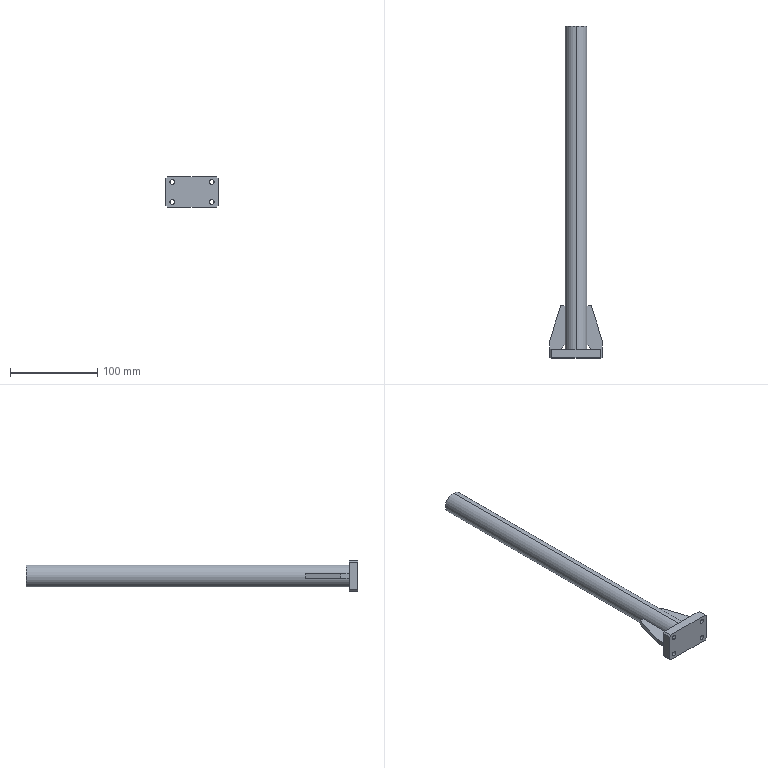Part | SolidWorks | features HoleWzd 2, ICE 2, Chamfer 1, Extrusion 1 | 4 solids | 42 faces | box 60 x 380 x 35 mm | volume 206976 mm3 | plane 28 | cylinder 12 | cone 2 | commonest cylinder face diameters 5.5 x8 6.8 x2 25 x2
STEP:
#1=CARTESIAN_POINT('',(17.5,0.,-2.5));
#2=VERTEX_POINT('',#1);
#3=CARTESIAN_POINT('',(30.,0.,-2.5));
#4=VERTEX_POINT('',#3);
#5=CARTESIAN_POINT('',(17.5,0.,-2.5));
#6=DIRECTION('',(1.,0.,0.));
#7=VECTOR('',#6,1000.);
#8=LINE('',#5,#7);
#9=EDGE_CURVE('',#2,#4,#8,.T.);
#10=ORIENTED_EDGE('',*,*,#9,.T.);
#11=CARTESIAN_POINT('',(30.,0.,2.5));
#12=VERTEX_POINT('',#11);
#13=CARTESIAN_POINT('',(30.,0.,2.5));
#14=DIRECTION('',(0.,0.,-1.));
#15=VECTOR('',#14,1000.);
#16=LINE('',#13,#15);
#17=EDGE_CURVE('',#12,#4,#16,.T.);
#18=ORIENTED_EDGE('',*,*,#17,.F.);
#19=CARTESIAN_POINT('',(17.5,0.,2.5));
#20=VERTEX_POINT('',#19);
#21=CARTESIAN_POINT('',(17.5,0.,2.5));
#22=DIRECTION('',(1.,0.,0.));
#23=VECTOR('',#22,1000.);
#24=LINE('',#21,#23);
#25=EDGE_CURVE('',#20,#12,#24,.T.);
#26=ORIENTED_EDGE('',*,*,#25,.F.);
#27=CARTESIAN_POINT('',(17.5,0.,2.5));
#28=DIRECTION('',(0.,0.,-1.));
#29=VECTOR('',#28,1000.);
#30=LINE('',#27,#29);
#31=EDGE_CURVE('',#20,#2,#30,.T.);
#32=ORIENTED_EDGE('',*,*,#31,.T.);
#33=EDGE_LOOP('',(#10,#18,#26,#32));
#34=FACE_OUTER_BOUND('',#33,.T.);
#35=CARTESIAN_POINT('',(17.5,0.,2.5));
#36=DIRECTION('',(0.,1.,0.));
#37=DIRECTION('',(0.,0.,1.));
#38=AXIS2_PLACEMENT_3D('',#35,#36,#37);
#39=PLANE('',#38);
#40=ADVANCED_FACE('',(#34),#39,.F.);
#41=CARTESIAN_POINT('',(30.,10.,-2.5));
#42=VERTEX_POINT('',#41);
#43=CARTESIAN_POINT('',(30.,0.,-2.5));
#44=DIRECTION('',(0.,1.,0.));
#45=VECTOR('',#44,1000.);
#46=LINE('',#43,#45);
#47=EDGE_CURVE('',#4,#42,#46,.T.);
#48=ORIENTED_EDGE('',*,*,#47,.T.);
#49=CARTESIAN_POINT('',(30.,10.,2.5));
#50=VERTEX_POINT('',#49);
#51=CARTESIAN_POINT('',(30.,10.,2.5));
#52=DIRECTION('',(0.,0.,-1.));
#53=VECTOR('',#52,1000.);
#54=LINE('',#51,#53);
#55=EDGE_CURVE('',#50,#42,#54,.T.);
#56=ORIENTED_EDGE('',*,*,#55,.F.);
#57=CARTESIAN_POINT('',(30.,0.,2.5));
#58=DIRECTION('',(0.,1.,0.));
#59=VECTOR('',#58,1000.);
#60=LINE('',#57,#59);
#61=EDGE_CURVE('',#12,#50,#60,.T.);
#62=ORIENTED_EDGE('',*,*,#61,.F.);
#63=ORIENTED_EDGE('',*,*,#17,.T.);
#64=EDGE_LOOP('',(#48,#56,#62,#63));
#65=FACE_OUTER_BOUND('',#64,.T.);
#66=CARTESIAN_POINT('',(30.,0.,2.5));
#67=DIRECTION('',(-1.,0.,0.));
#68=DIRECTION('',(0.,0.,1.));
#69=AXIS2_PLACEMENT_3D('',#66,#67,#68);
#70=PLANE('',#69);
#71=ADVANCED_FACE('',(#65),#70,.F.);
#72=CARTESIAN_POINT('',(17.5,50.,-2.5));
#73=VERTEX_POINT('',#72);
#74=CARTESIAN_POINT('',(30.,10.,-2.5));
#75=DIRECTION('',(-0.2983,0.9545,0.));
#76=VECTOR('',#75,1000.);
#77=LINE('',#74,#76);
#78=EDGE_CURVE('',#42,#73,#77,.T.);
#79=ORIENTED_EDGE('',*,*,#78,.T.);
#80=CARTESIAN_POINT('',(17.5,50.,2.5));
#81=VERTEX_POINT('',#80);
#82=CARTESIAN_POINT('',(17.5,50.,2.5));
#83=DIRECTION('',(0.,0.,-1.));
#84=VECTOR('',#83,1000.);
#85=LINE('',#82,#84);
#86=EDGE_CURVE('',#81,#73,#85,.T.);
#87=ORIENTED_EDGE('',*,*,#86,.F.);
#88=CARTESIAN_POINT('',(30.,10.,2.5));
#89=DIRECTION('',(-0.2983,0.9545,0.));
#90=VECTOR('',#89,1000.);
#91=LINE('',#88,#90);
#92=EDGE_CURVE('',#50,#81,#91,.T.);
#93=ORIENTED_EDGE('',*,*,#92,.F.);
#94=ORIENTED_EDGE('',*,*,#55,.T.);
#95=EDGE_LOOP('',(#79,#87,#93,#94));
#96=FACE_OUTER_BOUND('',#95,.T.);
#97=CARTESIAN_POINT('',(30.,10.,2.5));
#98=DIRECTION('',(-0.9545,-0.2983,0.));
#99=DIRECTION('',(0.2983,-0.9545,0.));
#100=AXIS2_PLACEMENT_3D('',#97,#98,#99);
#101=PLANE('',#100);
#102=ADVANCED_FACE('',(#96),#101,.F.);
#103=CARTESIAN_POINT('',(12.5,50.,-2.5));
#104=VERTEX_POINT('',#103);
#105=CARTESIAN_POINT('',(17.5,50.,-2.5));
#106=DIRECTION('',(-1.,0.,0.));
#107=VECTOR('',#106,1000.);
#108=LINE('',#105,#107);
#109=EDGE_CURVE('',#73,#104,#108,.T.);
#110=ORIENTED_EDGE('',*,*,#109,.T.);
#111=CARTESIAN_POINT('',(12.5,50.,2.5));
#112=VERTEX_POINT('',#111);
#113=CARTESIAN_POINT('',(12.5,50.,2.5));
#114=DIRECTION('',(0.,0.,-1.));
#115=VECTOR('',#114,1000.);
#116=LINE('',#113,#115);
#117=EDGE_CURVE('',#112,#104,#116,.T.);
#118=ORIENTED_EDGE('',*,*,#117,.F.);
#119=CARTESIAN_POINT('',(17.5,50.,2.5));
#120=DIRECTION('',(-1.,0.,0.));
#121=VECTOR('',#120,1000.);
#122=LINE('',#119,#121);
#123=EDGE_CURVE('',#81,#112,#122,.T.);
#124=ORIENTED_EDGE('',*,*,#123,.F.);
#125=ORIENTED_EDGE('',*,*,#86,.T.);
#126=EDGE_LOOP('',(#110,#118,#124,#125));
#127=FACE_OUTER_BOUND('',#126,.T.);
#128=CARTESIAN_POINT('',(17.5,50.,2.5));
#129=DIRECTION('',(0.,-1.,0.));
#130=DIRECTION('',(0.,0.,-1.));
#131=AXIS2_PLACEMENT_3D('',#128,#129,#130);
#132=PLANE('',#131);
#133=ADVANCED_FACE('',(#127),#132,.F.);
#134=CARTESIAN_POINT('',(12.5,5.,-2.5));
#135=VERTEX_POINT('',#134);
#136=CARTESIAN_POINT('',(12.5,50.,-2.5));
#137=DIRECTION('',(0.,-1.,0.));
#138=VECTOR('',#137,1000.);
#139=LINE('',#136,#138);
#140=EDGE_CURVE('',#104,#135,#139,.T.);
#141=ORIENTED_EDGE('',*,*,#140,.T.);
#142=CARTESIAN_POINT('',(12.5,5.,2.5));
#143=VERTEX_POINT('',#142);
#144=CARTESIAN_POINT('',(12.5,5.,2.5));
#145=DIRECTION('',(0.,0.,-1.));
#146=VECTOR('',#145,1000.);
#147=LINE('',#144,#146);
#148=EDGE_CURVE('',#143,#135,#147,.T.);
#149=ORIENTED_EDGE('',*,*,#148,.F.);
#150=CARTESIAN_POINT('',(12.5,50.,2.5));
#151=DIRECTION('',(0.,-1.,0.));
#152=VECTOR('',#151,1000.);
#153=LINE('',#150,#152);
#154=EDGE_CURVE('',#112,#143,#153,.T.);
#155=ORIENTED_EDGE('',*,*,#154,.F.);
#156=ORIENTED_EDGE('',*,*,#117,.T.);
#157=EDGE_LOOP('',(#141,#149,#155,#156));
#158=FACE_OUTER_BOUND('',#157,.T.);
#159=CARTESIAN_POINT('',(12.5,50.,2.5));
#160=DIRECTION('',(1.,0.,0.));
#161=DIRECTION('',(0.,1.,0.));
#162=AXIS2_PLACEMENT_3D('',#159,#160,#161);
#163=PLANE('',#162);
#164=ADVANCED_FACE('',(#158),#163,.F.);
#165=CARTESIAN_POINT('',(12.5,5.,-2.5));
#166=DIRECTION('',(0.7071,-0.7071,0.));
#167=VECTOR('',#166,1000.);
#168=LINE('',#165,#167);
#169=EDGE_CURVE('',#135,#2,#168,.T.);
#170=ORIENTED_EDGE('',*,*,#169,.T.);
#171=ORIENTED_EDGE('',*,*,#31,.F.);
#172=CARTESIAN_POINT('',(12.5,5.,2.5));
#173=DIRECTION('',(0.7071,-0.7071,0.));
#174=VECTOR('',#173,1000.);
#175=LINE('',#172,#174);
#176=EDGE_CURVE('',#143,#20,#175,.T.);
#177=ORIENTED_EDGE('',*,*,#176,.F.);
#178=ORIENTED_EDGE('',*,*,#148,.T.);
#179=EDGE_LOOP('',(#170,#171,#177,#178));
#180=FACE_OUTER_BOUND('',#179,.T.);
#181=CARTESIAN_POINT('',(12.5,5.,2.5));
#182=DIRECTION('',(0.7071,0.7071,0.));
#183=DIRECTION('',(-0.7071,0.7071,0.));
#184=AXIS2_PLACEMENT_3D('',#181,#182,#183);
#185=PLANE('',#184);
#186=ADVANCED_FACE('',(#180),#185,.F.);
#187=ORIENTED_EDGE('',*,*,#25,.T.);
#188=ORIENTED_EDGE('',*,*,#61,.T.);
#189=ORIENTED_EDGE('',*,*,#92,.T.);
#190=ORIENTED_EDGE('',*,*,#123,.T.);
#191=ORIENTED_EDGE('',*,*,#154,.T.);
#192=ORIENTED_EDGE('',*,*,#176,.T.);
#193=EDGE_LOOP('',(#187,#188,#189,#190,#191,#192));
#194=FACE_OUTER_BOUND('',#193,.T.);
#195=CARTESIAN_POINT('',(0.,0.,2.5));
#196=DIRECTION('',(0.,0.,1.));
#197=DIRECTION('',(1.,0.,0.));
#198=AXIS2_PLACEMENT_3D('',#195,#196,#197);
#199=PLANE('',#198);
#200=ADVANCED_FACE('',(#194),#199,.T.);
#201=ORIENTED_EDGE('',*,*,#9,.F.);
#202=ORIENTED_EDGE('',*,*,#169,.F.);
#203=ORIENTED_EDGE('',*,*,#140,.F.);
#204=ORIENTED_EDGE('',*,*,#109,.F.);
#205=ORIENTED_EDGE('',*,*,#78,.F.);
#206=ORIENTED_EDGE('',*,*,#47,.F.);
#207=EDGE_LOOP('',(#201,#202,#203,#204,#205,#206));
#208=FACE_OUTER_BOUND('',#207,.T.);
#209=CARTESIAN_POINT('',(0.,0.,-2.5));
#210=DIRECTION('',(0.,0.,1.));
#211=DIRECTION('',(1.,0.,0.));
#212=AXIS2_PLACEMENT_3D('',#209,#210,#211);
#213=PLANE('',#212);
#214=ADVANCED_FACE('',(#208),#213,.F.);
#215=CLOSED_SHELL('',(#40,#71,#102,#133,#164,#186,#200,#214));
#216=MANIFOLD_SOLID_BREP('',#215);
#217=CARTESIAN_POINT('',(-12.5,5.,-2.5));
#218=VERTEX_POINT('',#217);
#219=CARTESIAN_POINT('',(-12.5,50.,-2.5));
#220=VERTEX_POINT('',#219);
#221=CARTESIAN_POINT('',(-12.5,50.,-2.5));
#222=DIRECTION('',(0.,1.,0.));
#223=VECTOR('',#222,1000.);
#224=LINE('',#221,#223);
#225=EDGE_CURVE('',#218,#220,#224,.T.);
#226=ORIENTED_EDGE('',*,*,#225,.T.);
#227=CARTESIAN_POINT('',(-12.5,50.,2.5));
#228=VERTEX_POINT('',#227);
#229=CARTESIAN_POINT('',(-12.5,50.,2.5));
#230=DIRECTION('',(0.,0.,-1.));
#231=VECTOR('',#230,1000.);
#232=LINE('',#229,#231);
#233=EDGE_CURVE('',#228,#220,#232,.T.);
#234=ORIENTED_EDGE('',*,*,#233,.F.);
#235=CARTESIAN_POINT('',(-12.5,5.,2.5));
#236=VERTEX_POINT('',#235);
#237=CARTESIAN_POINT('',(-12.5,50.,2.5));
#238=DIRECTION('',(0.,1.,0.));
#239=VECTOR('',#238,1000.);
#240=LINE('',#237,#239);
#241=EDGE_CURVE('',#236,#228,#240,.T.);
#242=ORIENTED_EDGE('',*,*,#241,.F.);
#243=CARTESIAN_POINT('',(-12.5,5.,2.5));
#244=DIRECTION('',(0.,0.,-1.));
#245=VECTOR('',#244,1000.);
#246=LINE('',#243,#245);
#247=EDGE_CURVE('',#236,#218,#246,.T.);
#248=ORIENTED_EDGE('',*,*,#247,.T.);
#249=EDGE_LOOP('',(#226,#234,#242,#248));
#250=FACE_OUTER_BOUND('',#249,.T.);
#251=CARTESIAN_POINT('',(-12.5,50.,2.5));
#252=DIRECTION('',(-1.,0.,0.));
#253=DIRECTION('',(0.,-1.,0.));
#254=AXIS2_PLACEMENT_3D('',#251,#252,#253);
#255=PLANE('',#254);
#256=ADVANCED_FACE('',(#250),#255,.F.);
#257=CARTESIAN_POINT('',(-17.5,50.,-2.5));
#258=VERTEX_POINT('',#257);
#259=CARTESIAN_POINT('',(-17.5,50.,-2.5));
#260=DIRECTION('',(-1.,0.,0.));
#261=VECTOR('',#260,1000.);
#262=LINE('',#259,#261);
#263=EDGE_CURVE('',#220,#258,#262,.T.);
#264=ORIENTED_EDGE('',*,*,#263,.T.);
#265=CARTESIAN_POINT('',(-17.5,50.,2.5));
#266=VERTEX_POINT('',#265);
#267=CARTESIAN_POINT('',(-17.5,50.,2.5));
#268=DIRECTION('',(0.,0.,-1.));
#269=VECTOR('',#268,1000.);
#270=LINE('',#267,#269);
#271=EDGE_CURVE('',#266,#258,#270,.T.);
#272=ORIENTED_EDGE('',*,*,#271,.F.);
#273=CARTESIAN_POINT('',(-17.5,50.,2.5));
#274=DIRECTION('',(-1.,0.,0.));
#275=VECTOR('',#274,1000.);
#276=LINE('',#273,#275);
#277=EDGE_CURVE('',#228,#266,#276,.T.);
#278=ORIENTED_EDGE('',*,*,#277,.F.);
#279=ORIENTED_EDGE('',*,*,#233,.T.);
#280=EDGE_LOOP('',(#264,#272,#278,#279));
#281=FACE_OUTER_BOUND('',#280,.T.);
#282=CARTESIAN_POINT('',(-17.5,50.,2.5));
#283=DIRECTION('',(0.,-1.,0.));
#284=DIRECTION('',(1.,0.,0.));
#285=AXIS2_PLACEMENT_3D('',#282,#283,#284);
#286=PLANE('',#285);
#287=ADVANCED_FACE('',(#281),#286,.F.);
#288=CARTESIAN_POINT('',(-30.,10.,-2.5));
#289=VERTEX_POINT('',#288);
#290=CARTESIAN_POINT('',(-30.,10.,-2.5));
#291=DIRECTION('',(-0.2983,-0.9545,0.));
#292=VECTOR('',#291,1000.);
#293=LINE('',#290,#292);
#294=EDGE_CURVE('',#258,#289,#293,.T.);
#295=ORIENTED_EDGE('',*,*,#294,.T.);
#296=CARTESIAN_POINT('',(-30.,10.,2.5));
#297=VERTEX_POINT('',#296);
#298=CARTESIAN_POINT('',(-30.,10.,2.5));
#299=DIRECTION('',(0.,0.,-1.));
#300=VECTOR('',#299,1000.);
#301=LINE('',#298,#300);
#302=EDGE_CURVE('',#297,#289,#301,.T.);
#303=ORIENTED_EDGE('',*,*,#302,.F.);
#304=CARTESIAN_POINT('',(-30.,10.,2.5));
#305=DIRECTION('',(-0.2983,-0.9545,0.));
#306=VECTOR('',#305,1000.);
#307=LINE('',#304,#306);
#308=EDGE_CURVE('',#266,#297,#307,.T.);
#309=ORIENTED_EDGE('',*,*,#308,.F.);
#310=ORIENTED_EDGE('',*,*,#271,.T.);
#311=EDGE_LOOP('',(#295,#303,#309,#310));
#312=FACE_OUTER_BOUND('',#311,.T.);
#313=CARTESIAN_POINT('',(-30.,10.,2.5));
#314=DIRECTION('',(0.9545,-0.2983,0.));
#315=DIRECTION('',(0.2983,0.9545,0.));
#316=AXIS2_PLACEMENT_3D('',#313,#314,#315);
#317=PLANE('',#316);
#318=ADVANCED_FACE('',(#312),#317,.F.);
#319=CARTESIAN_POINT('',(-30.,0.,-2.5));
#320=VERTEX_POINT('',#319);
#321=CARTESIAN_POINT('',(-30.,0.,-2.5));
#322=DIRECTION('',(0.,-1.,0.));
#323=VECTOR('',#322,1000.);
#324=LINE('',#321,#323);
#325=EDGE_CURVE('',#289,#320,#324,.T.);
#326=ORIENTED_EDGE('',*,*,#325,.T.);
#327=CARTESIAN_POINT('',(-30.,0.,2.5));
#328=VERTEX_POINT('',#327);
#329=CARTESIAN_POINT('',(-30.,0.,2.5));
#330=DIRECTION('',(0.,0.,-1.));
#331=VECTOR('',#330,1000.);
#332=LINE('',#329,#331);
#333=EDGE_CURVE('',#328,#320,#332,.T.);
#334=ORIENTED_EDGE('',*,*,#333,.F.);
#335=CARTESIAN_POINT('',(-30.,0.,2.5));
#336=DIRECTION('',(0.,-1.,0.));
#337=VECTOR('',#336,1000.);
#338=LINE('',#335,#337);
#339=EDGE_CURVE('',#297,#328,#338,.T.);
#340=ORIENTED_EDGE('',*,*,#339,.F.);
#341=ORIENTED_EDGE('',*,*,#302,.T.);
#342=EDGE_LOOP('',(#326,#334,#340,#341));
#343=FACE_OUTER_BOUND('',#342,.T.);
#344=CARTESIAN_POINT('',(-30.,0.,2.5));
#345=DIRECTION('',(1.,0.,0.));
#346=DIRECTION('',(0.,0.,-1.));
#347=AXIS2_PLACEMENT_3D('',#344,#345,#346);
#348=PLANE('',#347);
#349=ADVANCED_FACE('',(#343),#348,.F.);
#350=CARTESIAN_POINT('',(-17.5,0.,-2.5));
#351=VERTEX_POINT('',#350);
#352=CARTESIAN_POINT('',(-17.5,0.,-2.5));
#353=DIRECTION('',(1.,0.,0.));
#354=VECTOR('',#353,1000.);
#355=LINE('',#352,#354);
#356=EDGE_CURVE('',#320,#351,#355,.T.);
#357=ORIENTED_EDGE('',*,*,#356,.T.);
#358=CARTESIAN_POINT('',(-17.5,0.,2.5));
#359=VERTEX_POINT('',#358);
#360=CARTESIAN_POINT('',(-17.5,0.,2.5));
#361=DIRECTION('',(0.,0.,-1.));
#362=VECTOR('',#361,1000.);
#363=LINE('',#360,#362);
#364=EDGE_CURVE('',#359,#351,#363,.T.);
#365=ORIENTED_EDGE('',*,*,#364,.F.);
#366=CARTESIAN_POINT('',(-17.5,0.,2.5));
#367=DIRECTION('',(1.,0.,0.));
#368=VECTOR('',#367,1000.);
#369=LINE('',#366,#368);
#370=EDGE_CURVE('',#328,#359,#369,.T.);
#371=ORIENTED_EDGE('',*,*,#370,.F.);
#372=ORIENTED_EDGE('',*,*,#333,.T.);
#373=EDGE_LOOP('',(#357,#365,#371,#372));
#374=FACE_OUTER_BOUND('',#373,.T.);
#375=CARTESIAN_POINT('',(-17.5,0.,2.5));
#376=DIRECTION('',(0.,1.,0.));
#377=DIRECTION('',(0.,0.,1.));
#378=AXIS2_PLACEMENT_3D('',#375,#376,#377);
#379=PLANE('',#378);
#380=ADVANCED_FACE('',(#374),#379,.F.);
#381=CARTESIAN_POINT('',(-12.5,5.,-2.5));
#382=DIRECTION('',(0.7071,0.7071,0.));
#383=VECTOR('',#382,1000.);
#384=LINE('',#381,#383);
#385=EDGE_CURVE('',#351,#218,#384,.T.);
#386=ORIENTED_EDGE('',*,*,#385,.T.);
#387=ORIENTED_EDGE('',*,*,#247,.F.);
#388=CARTESIAN_POINT('',(-12.5,5.,2.5));
#389=DIRECTION('',(0.7071,0.7071,0.));
#390=VECTOR('',#389,1000.);
#391=LINE('',#388,#390);
#392=EDGE_CURVE('',#359,#236,#391,.T.);
#393=ORIENTED_EDGE('',*,*,#392,.F.);
#394=ORIENTED_EDGE('',*,*,#364,.T.);
#395=EDGE_LOOP('',(#386,#387,#393,#394));
#396=FACE_OUTER_BOUND('',#395,.T.);
#397=CARTESIAN_POINT('',(-12.5,5.,2.5));
#398=DIRECTION('',(-0.7071,0.7071,0.));
#399=DIRECTION('',(-0.7071,-0.7071,0.));
#400=AXIS2_PLACEMENT_3D('',#397,#398,#399);
#401=PLANE('',#400);
#402=ADVANCED_FACE('',(#396),#401,.F.);
#403=ORIENTED_EDGE('',*,*,#241,.T.);
#404=ORIENTED_EDGE('',*,*,#277,.T.);
#405=ORIENTED_EDGE('',*,*,#308,.T.);
#406=ORIENTED_EDGE('',*,*,#339,.T.);
#407=ORIENTED_EDGE('',*,*,#370,.T.);
#408=ORIENTED_EDGE('',*,*,#392,.T.);
#409=EDGE_LOOP('',(#403,#404,#405,#406,#407,#408));
#410=FACE_OUTER_BOUND('',#409,.T.);
#411=CARTESIAN_POINT('',(0.,0.,2.5));
#412=DIRECTION('',(0.,0.,-1.));
#413=DIRECTION('',(-1.,0.,0.));
#414=AXIS2_PLACEMENT_3D('',#411,#412,#413);
#415=PLANE('',#414);
#416=ADVANCED_FACE('',(#410),#415,.F.);
#417=ORIENTED_EDGE('',*,*,#225,.F.);
#418=ORIENTED_EDGE('',*,*,#385,.F.);
#419=ORIENTED_EDGE('',*,*,#356,.F.);
#420=ORIENTED_EDGE('',*,*,#325,.F.);
#421=ORIENTED_EDGE('',*,*,#294,.F.);
#422=ORIENTED_EDGE('',*,*,#263,.F.);
#423=EDGE_LOOP('',(#417,#418,#419,#420,#421,#422));
#424=FACE_OUTER_BOUND('',#423,.T.);
#425=CARTESIAN_POINT('',(0.,0.,-2.5));
#426=DIRECTION('',(0.,0.,-1.));
#427=DIRECTION('',(-1.,0.,0.));
#428=AXIS2_PLACEMENT_3D('',#425,#426,#427);
#429=PLANE('',#428);
#430=ADVANCED_FACE('',(#424),#429,.T.);
#431=CLOSED_SHELL('',(#256,#287,#318,#349,#380,#402,#416,#430));
#432=MANIFOLD_SOLID_BREP('',#431);
#433=CARTESIAN_POINT('',(22.5,0.,14.25));
#434=VERTEX_POINT('',#433);
#435=CARTESIAN_POINT('',(22.5,0.,8.75));
#436=VERTEX_POINT('',#435);
#437=CARTESIAN_POINT('',(22.5,0.,11.5));
#438=DIRECTION('',(0.,-1.,0.));
#439=DIRECTION('',(0.,0.,-1.));
#440=AXIS2_PLACEMENT_3D('',#437,#438,#439);
#441=CIRCLE('',#440,2.75);
#442=EDGE_CURVE('',#434,#436,#441,.T.);
#443=ORIENTED_EDGE('',*,*,#442,.F.);
#444=CARTESIAN_POINT('',(22.5,-10.,14.25));
#445=VERTEX_POINT('',#444);
#446=CARTESIAN_POINT('',(22.5,-10.,14.25));
#447=DIRECTION('',(0.,-1.,0.));
#448=VECTOR('',#447,1000.);
#449=LINE('',#446,#448);
#450=EDGE_CURVE('',#434,#445,#449,.T.);
#451=ORIENTED_EDGE('',*,*,#450,.T.);
#452=CARTESIAN_POINT('',(22.5,-10.,8.75));
#453=VERTEX_POINT('',#452);
#454=CARTESIAN_POINT('',(22.5,-10.,11.5));
#455=DIRECTION('',(0.,-1.,0.));
#456=DIRECTION('',(0.,0.,-1.));
#457=AXIS2_PLACEMENT_3D('',#454,#455,#456);
#458=CIRCLE('',#457,2.75);
#459=EDGE_CURVE('',#445,#453,#458,.T.);
#460=ORIENTED_EDGE('',*,*,#459,.T.);
#461=CARTESIAN_POINT('',(22.5,-10.,8.75));
#462=DIRECTION('',(0.,-1.,0.));
#463=VECTOR('',#462,1000.);
#464=LINE('',#461,#463);
#465=EDGE_CURVE('',#436,#453,#464,.T.);
#466=ORIENTED_EDGE('',*,*,#465,.F.);
#467=EDGE_LOOP('',(#443,#451,#460,#466));
#468=FACE_OUTER_BOUND('',#467,.T.);
#469=CARTESIAN_POINT('',(22.5,-10.,11.5));
#470=DIRECTION('',(0.,-1.,0.));
#471=DIRECTION('',(0.,0.,-1.));
#472=AXIS2_PLACEMENT_3D('',#469,#470,#471);
#473=CYLINDRICAL_SURFACE('',#472,2.75);
#474=ADVANCED_FACE('',(#468),#473,.F.);
#475=CARTESIAN_POINT('',(22.5,0.,-8.75));
#476=VERTEX_POINT('',#475);
#477=CARTESIAN_POINT('',(22.5,0.,-14.25));
#478=VERTEX_POINT('',#477);
#479=CARTESIAN_POINT('',(22.5,0.,-11.5));
#480=DIRECTION('',(0.,-1.,0.));
#481=DIRECTION('',(0.,0.,-1.));
#482=AXIS2_PLACEMENT_3D('',#479,#480,#481);
#483=CIRCLE('',#482,2.75);
#484=EDGE_CURVE('',#476,#478,#483,.T.);
#485=ORIENTED_EDGE('',*,*,#484,.F.);
#486=CARTESIAN_POINT('',(22.5,-10.,-8.75));
#487=VERTEX_POINT('',#486);
#488=CARTESIAN_POINT('',(22.5,-10.,-8.75));
#489=DIRECTION('',(0.,-1.,0.));
#490=VECTOR('',#489,1000.);
#491=LINE('',#488,#490);
#492=EDGE_CURVE('',#476,#487,#491,.T.);
#493=ORIENTED_EDGE('',*,*,#492,.T.);
#494=CARTESIAN_POINT('',(22.5,-10.,-14.25));
#495=VERTEX_POINT('',#494);
#496=CARTESIAN_POINT('',(22.5,-10.,-11.5));
#497=DIRECTION('',(0.,-1.,0.));
#498=DIRECTION('',(0.,0.,-1.));
#499=AXIS2_PLACEMENT_3D('',#496,#497,#498);
#500=CIRCLE('',#499,2.75);
#501=EDGE_CURVE('',#487,#495,#500,.T.);
#502=ORIENTED_EDGE('',*,*,#501,.T.);
#503=CARTESIAN_POINT('',(22.5,-10.,-14.25));
#504=DIRECTION('',(0.,-1.,0.));
#505=VECTOR('',#504,1000.);
#506=LINE('',#503,#505);
#507=EDGE_CURVE('',#478,#495,#506,.T.);
#508=ORIENTED_EDGE('',*,*,#507,.F.);
#509=EDGE_LOOP('',(#485,#493,#502,#508));
#510=FACE_OUTER_BOUND('',#509,.T.);
#511=CARTESIAN_POINT('',(22.5,-10.,-11.5));
#512=DIRECTION('',(0.,-1.,0.));
#513=DIRECTION('',(0.,0.,-1.));
#514=AXIS2_PLACEMENT_3D('',#511,#512,#513);
#515=CYLINDRICAL_SURFACE('',#514,2.75);
#516=ADVANCED_FACE('',(#510),#515,.F.);
#517=CARTESIAN_POINT('',(-22.5,0.,-8.75));
#518=VERTEX_POINT('',#517);
#519=CARTESIAN_POINT('',(-22.5,0.,-14.25));
#520=VERTEX_POINT('',#519);
#521=CARTESIAN_POINT('',(-22.5,0.,-11.5));
#522=DIRECTION('',(0.,-1.,0.));
#523=DIRECTION('',(0.,0.,-1.));
#524=AXIS2_PLACEMENT_3D('',#521,#522,#523);
#525=CIRCLE('',#524,2.75);
#526=EDGE_CURVE('',#518,#520,#525,.T.);
#527=ORIENTED_EDGE('',*,*,#526,.F.);
#528=CARTESIAN_POINT('',(-22.5,-10.,-8.75));
#529=VERTEX_POINT('',#528);
#530=CARTESIAN_POINT('',(-22.5,-10.,-8.75));
#531=DIRECTION('',(0.,-1.,0.));
#532=VECTOR('',#531,1000.);
#533=LINE('',#530,#532);
#534=EDGE_CURVE('',#518,#529,#533,.T.);
#535=ORIENTED_EDGE('',*,*,#534,.T.);
#536=CARTESIAN_POINT('',(-22.5,-10.,-14.25));
#537=VERTEX_POINT('',#536);
#538=CARTESIAN_POINT('',(-22.5,-10.,-11.5));
#539=DIRECTION('',(0.,-1.,0.));
#540=DIRECTION('',(0.,0.,-1.));
#541=AXIS2_PLACEMENT_3D('',#538,#539,#540);
#542=CIRCLE('',#541,2.75);
#543=EDGE_CURVE('',#529,#537,#542,.T.);
#544=ORIENTED_EDGE('',*,*,#543,.T.);
#545=CARTESIAN_POINT('',(-22.5,-10.,-14.25));
#546=DIRECTION('',(0.,-1.,0.));
#547=VECTOR('',#546,1000.);
#548=LINE('',#545,#547);
#549=EDGE_CURVE('',#520,#537,#548,.T.);
#550=ORIENTED_EDGE('',*,*,#549,.F.);
#551=EDGE_LOOP('',(#527,#535,#544,#550));
#552=FACE_OUTER_BOUND('',#551,.T.);
#553=CARTESIAN_POINT('',(-22.5,-10.,-11.5));
#554=DIRECTION('',(0.,-1.,0.));
#555=DIRECTION('',(0.,0.,-1.));
#556=AXIS2_PLACEMENT_3D('',#553,#554,#555);
#557=CYLINDRICAL_SURFACE('',#556,2.75);
#558=ADVANCED_FACE('',(#552),#557,.F.);
#559=CARTESIAN_POINT('',(-22.5,0.,14.25));
#560=VERTEX_POINT('',#559);
#561=CARTESIAN_POINT('',(-22.5,0.,8.75));
#562=VERTEX_POINT('',#561);
#563=CARTESIAN_POINT('',(-22.5,0.,11.5));
#564=DIRECTION('',(0.,-1.,0.));
#565=DIRECTION('',(0.,0.,-1.));
#566=AXIS2_PLACEMENT_3D('',#563,#564,#565);
#567=CIRCLE('',#566,2.75);
#568=EDGE_CURVE('',#560,#562,#567,.T.);
#569=ORIENTED_EDGE('',*,*,#568,.F.);
#570=CARTESIAN_POINT('',(-22.5,-10.,14.25));
#571=VERTEX_POINT('',#570);
#572=CARTESIAN_POINT('',(-22.5,-10.,14.25));
#573=DIRECTION('',(0.,-1.,0.));
#574=VECTOR('',#573,1000.);
#575=LINE('',#572,#574);
#576=EDGE_CURVE('',#560,#571,#575,.T.);
#577=ORIENTED_EDGE('',*,*,#576,.T.);
#578=CARTESIAN_POINT('',(-22.5,-10.,8.75));
#579=VERTEX_POINT('',#578);
#580=CARTESIAN_POINT('',(-22.5,-10.,11.5));
#581=DIRECTION('',(0.,-1.,0.));
#582=DIRECTION('',(0.,0.,-1.));
#583=AXIS2_PLACEMENT_3D('',#580,#581,#582);
#584=CIRCLE('',#583,2.75);
#585=EDGE_CURVE('',#571,#579,#584,.T.);
#586=ORIENTED_EDGE('',*,*,#585,.T.);
#587=CARTESIAN_POINT('',(-22.5,-10.,8.75));
#588=DIRECTION('',(0.,-1.,0.));
#589=VECTOR('',#588,1000.);
#590=LINE('',#587,#589);
#591=EDGE_CURVE('',#562,#579,#590,.T.);
#592=ORIENTED_EDGE('',*,*,#591,.F.);
#593=EDGE_LOOP('',(#569,#577,#586,#592));
#594=FACE_OUTER_BOUND('',#593,.T.);
#595=CARTESIAN_POINT('',(-22.5,-10.,11.5));
#596=DIRECTION('',(0.,-1.,0.));
#597=DIRECTION('',(0.,0.,-1.));
#598=AXIS2_PLACEMENT_3D('',#595,#596,#597);
#599=CYLINDRICAL_SURFACE('',#598,2.75);
#600=ADVANCED_FACE('',(#594),#599,.F.);
#601=CARTESIAN_POINT('',(-30.,0.,15.5));
#602=VERTEX_POINT('',#601);
#603=CARTESIAN_POINT('',(-30.,0.,-15.5));
#604=VERTEX_POINT('',#603);
#605=CARTESIAN_POINT('',(-30.,0.,-17.5));
#606=DIRECTION('',(0.,0.,-1.));
#607=VECTOR('',#606,1000.);
#608=LINE('',#605,#607);
#609=EDGE_CURVE('',#602,#604,#608,.T.);
#610=ORIENTED_EDGE('',*,*,#609,.T.);
#611=CARTESIAN_POINT('',(-30.,-10.,-15.5));
#612=VERTEX_POINT('',#611);
#613=CARTESIAN_POINT('',(-30.,-10.,-15.5));
#614=DIRECTION('',(0.,-1.,0.));
#615=VECTOR('',#614,1000.);
#616=LINE('',#613,#615);
#617=EDGE_CURVE('',#604,#612,#616,.T.);
#618=ORIENTED_EDGE('',*,*,#617,.T.);
#619=CARTESIAN_POINT('',(-30.,-10.,15.5));
#620=VERTEX_POINT('',#619);
#621=CARTESIAN_POINT('',(-30.,-10.,-17.5));
#622=DIRECTION('',(0.,0.,-1.));
#623=VECTOR('',#622,1000.);
#624=LINE('',#621,#623);
#625=EDGE_CURVE('',#620,#612,#624,.T.);
#626=ORIENTED_EDGE('',*,*,#625,.F.);
#627=CARTESIAN_POINT('',(-30.,-10.,15.5));
#628=DIRECTION('',(0.,1.,0.));
#629=VECTOR('',#628,1000.);
#630=LINE('',#627,#629);
#631=EDGE_CURVE('',#620,#602,#630,.T.);
#632=ORIENTED_EDGE('',*,*,#631,.T.);
#633=EDGE_LOOP('',(#610,#618,#626,#632));
#634=FACE_OUTER_BOUND('',#633,.T.);
#635=CARTESIAN_POINT('',(-30.,-10.,-17.5));
#636=DIRECTION('',(1.,0.,0.));
#637=DIRECTION('',(0.,0.,-1.));
#638=AXIS2_PLACEMENT_3D('',#635,#636,#637);
#639=PLANE('',#638);
#640=ADVANCED_FACE('',(#634),#639,.F.);
#641=CARTESIAN_POINT('',(-28.,-10.,-17.5));
#642=VERTEX_POINT('',#641);
#643=CARTESIAN_POINT('',(28.,-10.,-17.5));
#644=VERTEX_POINT('',#643);
#645=CARTESIAN_POINT('',(30.,-10.,-17.5));
#646=DIRECTION('',(1.,0.,0.));
#647=VECTOR('',#646,1000.);
#648=LINE('',#645,#647);
#649=EDGE_CURVE('',#642,#644,#648,.T.);
#650=ORIENTED_EDGE('',*,*,#649,.F.);
#651=CARTESIAN_POINT('',(-28.,0.,-17.5));
#652=VERTEX_POINT('',#651);
#653=CARTESIAN_POINT('',(-28.,-10.,-17.5));
#654=DIRECTION('',(0.,1.,0.));
#655=VECTOR('',#654,1000.);
#656=LINE('',#653,#655);
#657=EDGE_CURVE('',#642,#652,#656,.T.);
#658=ORIENTED_EDGE('',*,*,#657,.T.);
#659=CARTESIAN_POINT('',(28.,0.,-17.5));
#660=VERTEX_POINT('',#659);
#661=CARTESIAN_POINT('',(30.,0.,-17.5));
#662=DIRECTION('',(1.,0.,0.));
#663=VECTOR('',#662,1000.);
#664=LINE('',#661,#663);
#665=EDGE_CURVE('',#652,#660,#664,.T.);
#666=ORIENTED_EDGE('',*,*,#665,.T.);
#667=CARTESIAN_POINT('',(28.,-10.,-17.5));
#668=DIRECTION('',(0.,-1.,0.));
#669=VECTOR('',#668,1000.);
#670=LINE('',#667,#669);
#671=EDGE_CURVE('',#660,#644,#670,.T.);
#672=ORIENTED_EDGE('',*,*,#671,.T.);
#673=EDGE_LOOP('',(#650,#658,#666,#672));
#674=FACE_OUTER_BOUND('',#673,.T.);
#675=CARTESIAN_POINT('',(30.,-10.,-17.5));
#676=DIRECTION('',(0.,0.,1.));
#677=DIRECTION('',(1.,0.,0.));
#678=AXIS2_PLACEMENT_3D('',#675,#676,#677);
#679=PLANE('',#678);
#680=ADVANCED_FACE('',(#674),#679,.F.);
#681=CARTESIAN_POINT('',(30.,-10.,-15.5));
#682=VERTEX_POINT('',#681);
#683=CARTESIAN_POINT('',(30.,-10.,15.5));
#684=VERTEX_POINT('',#683);
#685=CARTESIAN_POINT('',(30.,-10.,-17.5));
#686=DIRECTION('',(0.,0.,1.));
#687=VECTOR('',#686,1000.);
#688=LINE('',#685,#687);
#689=EDGE_CURVE('',#682,#684,#688,.T.);
#690=ORIENTED_EDGE('',*,*,#689,.F.);
#691=CARTESIAN_POINT('',(30.,0.,-15.5));
#692=VERTEX_POINT('',#691);
#693=CARTESIAN_POINT('',(30.,-10.,-15.5));
#694=DIRECTION('',(0.,1.,0.));
#695=VECTOR('',#694,1000.);
#696=LINE('',#693,#695);
#697=EDGE_CURVE('',#682,#692,#696,.T.);
#698=ORIENTED_EDGE('',*,*,#697,.T.);
#699=CARTESIAN_POINT('',(30.,0.,15.5));
#700=VERTEX_POINT('',#699);
#701=CARTESIAN_POINT('',(30.,0.,-17.5));
#702=DIRECTION('',(0.,0.,1.));
#703=VECTOR('',#702,1000.);
#704=LINE('',#701,#703);
#705=EDGE_CURVE('',#692,#700,#704,.T.);
#706=ORIENTED_EDGE('',*,*,#705,.T.);
#707=CARTESIAN_POINT('',(30.,-10.,15.5));
#708=DIRECTION('',(0.,-1.,0.));
#709=VECTOR('',#708,1000.);
#710=LINE('',#707,#709);
#711=EDGE_CURVE('',#700,#684,#710,.T.);
#712=ORIENTED_EDGE('',*,*,#711,.T.);
#713=EDGE_LOOP('',(#690,#698,#706,#712));
#714=FACE_OUTER_BOUND('',#713,.T.);
#715=CARTESIAN_POINT('',(30.,-10.,-17.5));
#716=DIRECTION('',(-1.,0.,0.));
#717=DIRECTION('',(0.,0.,1.));
#718=AXIS2_PLACEMENT_3D('',#715,#716,#717);
#719=PLANE('',#718);
#720=ADVANCED_FACE('',(#714),#719,.F.);
#721=CARTESIAN_POINT('',(28.,0.,17.5));
#722=VERTEX_POINT('',#721);
#723=CARTESIAN_POINT('',(-28.,0.,17.5));
#724=VERTEX_POINT('',#723);
#725=CARTESIAN_POINT('',(30.,0.,17.5));
#726=DIRECTION('',(-1.,0.,0.));
#727=VECTOR('',#726,1000.);
#728=LINE('',#725,#727);
#729=EDGE_CURVE('',#722,#724,#728,.T.);
#730=ORIENTED_EDGE('',*,*,#729,.T.);
#731=CARTESIAN_POINT('',(-28.,-10.,17.5));
#732=VERTEX_POINT('',#731);
#733=CARTESIAN_POINT('',(-28.,-10.,17.5));
#734=DIRECTION('',(0.,-1.,0.));
#735=VECTOR('',#734,1000.);
#736=LINE('',#733,#735);
#737=EDGE_CURVE('',#724,#732,#736,.T.);
#738=ORIENTED_EDGE('',*,*,#737,.T.);
#739=CARTESIAN_POINT('',(28.,-10.,17.5));
#740=VERTEX_POINT('',#739);
#741=CARTESIAN_POINT('',(30.,-10.,17.5));
#742=DIRECTION('',(-1.,0.,0.));
#743=VECTOR('',#742,1000.);
#744=LINE('',#741,#743);
#745=EDGE_CURVE('',#740,#732,#744,.T.);
#746=ORIENTED_EDGE('',*,*,#745,.F.);
#747=CARTESIAN_POINT('',(28.,-10.,17.5));
#748=DIRECTION('',(0.,1.,0.));
#749=VECTOR('',#748,1000.);
#750=LINE('',#747,#749);
#751=EDGE_CURVE('',#740,#722,#750,.T.);
#752=ORIENTED_EDGE('',*,*,#751,.T.);
#753=EDGE_LOOP('',(#730,#738,#746,#752));
#754=FACE_OUTER_BOUND('',#753,.T.);
#755=CARTESIAN_POINT('',(30.,-10.,17.5));
#756=DIRECTION('',(0.,0.,-1.));
#757=DIRECTION('',(-1.,0.,0.));
#758=AXIS2_PLACEMENT_3D('',#755,#756,#757);
#759=PLANE('',#758);
#760=ADVANCED_FACE('',(#754),#759,.F.);
#761=CARTESIAN_POINT('',(22.5,-10.,11.5));
#762=DIRECTION('',(0.,-1.,0.));
#763=DIRECTION('',(0.,0.,-1.));
#764=AXIS2_PLACEMENT_3D('',#761,#762,#763);
#765=CIRCLE('',#764,2.75);
#766=EDGE_CURVE('',#453,#445,#765,.T.);
#767=ORIENTED_EDGE('',*,*,#766,.F.);
#768=ORIENTED_EDGE('',*,*,#459,.F.);
#769=EDGE_LOOP('',(#767,#768));
#770=FACE_BOUND('',#769,.T.);
#771=CARTESIAN_POINT('',(22.5,-10.,-11.5));
#772=DIRECTION('',(0.,-1.,0.));
#773=DIRECTION('',(0.,0.,-1.));
#774=AXIS2_PLACEMENT_3D('',#771,#772,#773);
#775=CIRCLE('',#774,2.75);
#776=EDGE_CURVE('',#495,#487,#775,.T.);
#777=ORIENTED_EDGE('',*,*,#776,.F.);
#778=ORIENTED_EDGE('',*,*,#501,.F.);
#779=EDGE_LOOP('',(#777,#778));
#780=FACE_BOUND('',#779,.T.);
#781=CARTESIAN_POINT('',(-22.5,-10.,-11.5));
#782=DIRECTION('',(0.,-1.,0.));
#783=DIRECTION('',(0.,0.,-1.));
#784=AXIS2_PLACEMENT_3D('',#781,#782,#783);
#785=CIRCLE('',#784,2.75);
#786=EDGE_CURVE('',#537,#529,#785,.T.);
#787=ORIENTED_EDGE('',*,*,#786,.F.);
#788=ORIENTED_EDGE('',*,*,#543,.F.);
#789=EDGE_LOOP('',(#787,#788));
#790=FACE_BOUND('',#789,.T.);
#791=CARTESIAN_POINT('',(-22.5,-10.,11.5));
#792=DIRECTION('',(0.,-1.,0.));
#793=DIRECTION('',(0.,0.,-1.));
#794=AXIS2_PLACEMENT_3D('',#791,#792,#793);
#795=CIRCLE('',#794,2.75);
#796=EDGE_CURVE('',#579,#571,#795,.T.);
#797=ORIENTED_EDGE('',*,*,#796,.F.);
#798=ORIENTED_EDGE('',*,*,#585,.F.);
#799=EDGE_LOOP('',(#797,#798));
#800=FACE_BOUND('',#799,.T.);
#801=ORIENTED_EDGE('',*,*,#625,.T.);
#802=CARTESIAN_POINT('',(-22.75,-10.,-22.75));
#803=DIRECTION('',(0.7071,0.,-0.7071));
#804=VECTOR('',#803,1000.);
#805=LINE('',#802,#804);
#806=EDGE_CURVE('',#612,#642,#805,.T.);
#807=ORIENTED_EDGE('',*,*,#806,.T.);
#808=ORIENTED_EDGE('',*,*,#649,.T.);
#809=CARTESIAN_POINT('',(22.75,-10.,-22.75));
#810=DIRECTION('',(0.7071,0.,0.7071));
#811=VECTOR('',#810,1000.);
#812=LINE('',#809,#811);
#813=EDGE_CURVE('',#644,#682,#812,.T.);
#814=ORIENTED_EDGE('',*,*,#813,.T.);
#815=ORIENTED_EDGE('',*,*,#689,.T.);
#816=CARTESIAN_POINT('',(22.75,-10.,22.75));
#817=DIRECTION('',(-0.7071,0.,0.7071));
#818=VECTOR('',#817,1000.);
#819=LINE('',#816,#818);
#820=EDGE_CURVE('',#684,#740,#819,.T.);
#821=ORIENTED_EDGE('',*,*,#820,.T.);
#822=ORIENTED_EDGE('',*,*,#745,.T.);
#823=CARTESIAN_POINT('',(-22.75,-10.,22.75));
#824=DIRECTION('',(-0.7071,0.,-0.7071));
#825=VECTOR('',#824,1000.);
#826=LINE('',#823,#825);
#827=EDGE_CURVE('',#732,#620,#826,.T.);
#828=ORIENTED_EDGE('',*,*,#827,.T.);
#829=EDGE_LOOP('',(#801,#807,#808,#814,#815,#821,#822,#828));
#830=FACE_OUTER_BOUND('',#829,.T.);
#831=CARTESIAN_POINT('',(0.,-10.,0.));
#832=DIRECTION('',(0.,-1.,0.));
#833=DIRECTION('',(0.,0.,-1.));
#834=AXIS2_PLACEMENT_3D('',#831,#832,#833);
#835=PLANE('',#834);
#836=ADVANCED_FACE('',(#770,#780,#790,#800,#830),#835,.T.);
#837=CARTESIAN_POINT('',(22.5,0.,11.5));
#838=DIRECTION('',(0.,-1.,0.));
#839=DIRECTION('',(0.,0.,-1.));
#840=AXIS2_PLACEMENT_3D('',#837,#838,#839);
#841=CIRCLE('',#840,2.75);
#842=EDGE_CURVE('',#436,#434,#841,.T.);
#843=ORIENTED_EDGE('',*,*,#842,.T.);
#844=ORIENTED_EDGE('',*,*,#442,.T.);
#845=EDGE_LOOP('',(#843,#844));
#846=FACE_BOUND('',#845,.T.);
#847=CARTESIAN_POINT('',(22.5,0.,-11.5));
#848=DIRECTION('',(0.,-1.,0.));
#849=DIRECTION('',(0.,0.,-1.));
#850=AXIS2_PLACEMENT_3D('',#847,#848,#849);
#851=CIRCLE('',#850,2.75);
#852=EDGE_CURVE('',#478,#476,#851,.T.);
#853=ORIENTED_EDGE('',*,*,#852,.T.);
#854=ORIENTED_EDGE('',*,*,#484,.T.);
#855=EDGE_LOOP('',(#853,#854));
#856=FACE_BOUND('',#855,.T.);
#857=CARTESIAN_POINT('',(-22.5,0.,-11.5));
#858=DIRECTION('',(0.,-1.,0.));
#859=DIRECTION('',(0.,0.,-1.));
#860=AXIS2_PLACEMENT_3D('',#857,#858,#859);
#861=CIRCLE('',#860,2.75);
#862=EDGE_CURVE('',#520,#518,#861,.T.);
#863=ORIENTED_EDGE('',*,*,#862,.T.);
#864=ORIENTED_EDGE('',*,*,#526,.T.);
#865=EDGE_LOOP('',(#863,#864));
#866=FACE_BOUND('',#865,.T.);
#867=CARTESIAN_POINT('',(-22.5,0.,11.5));
#868=DIRECTION('',(0.,-1.,0.));
#869=DIRECTION('',(0.,0.,-1.));
#870=AXIS2_PLACEMENT_3D('',#867,#868,#869);
#871=CIRCLE('',#870,2.75);
#872=EDGE_CURVE('',#562,#560,#871,.T.);
#873=ORIENTED_EDGE('',*,*,#872,.T.);
#874=ORIENTED_EDGE('',*,*,#568,.T.);
#875=EDGE_LOOP('',(#873,#874));
#876=FACE_BOUND('',#875,.T.);
#877=ORIENTED_EDGE('',*,*,#665,.F.);
#878=CARTESIAN_POINT('',(-28.,0.,-17.5));
#879=DIRECTION('',(-0.7071,0.,0.7071));
#880=VECTOR('',#879,1000.);
#881=LINE('',#878,#880);
#882=EDGE_CURVE('',#652,#604,#881,.T.);
#883=ORIENTED_EDGE('',*,*,#882,.T.);
#884=ORIENTED_EDGE('',*,*,#609,.F.);
#885=CARTESIAN_POINT('',(-30.,0.,15.5));
#886=DIRECTION('',(0.7071,0.,0.7071));
#887=VECTOR('',#886,1000.);
#888=LINE('',#885,#887);
#889=EDGE_CURVE('',#602,#724,#888,.T.);
#890=ORIENTED_EDGE('',*,*,#889,.T.);
#891=ORIENTED_EDGE('',*,*,#729,.F.);
#892=CARTESIAN_POINT('',(28.,0.,17.5));
#893=DIRECTION('',(0.7071,0.,-0.7071));
#894=VECTOR('',#893,1000.);
#895=LINE('',#892,#894);
#896=EDGE_CURVE('',#722,#700,#895,.T.);
#897=ORIENTED_EDGE('',*,*,#896,.T.);
#898=ORIENTED_EDGE('',*,*,#705,.F.);
#899=CARTESIAN_POINT('',(30.,0.,-15.5));
#900=DIRECTION('',(-0.7071,0.,-0.7071));
#901=VECTOR('',#900,1000.);
#902=LINE('',#899,#901);
#903=EDGE_CURVE('',#692,#660,#902,.T.);
#904=ORIENTED_EDGE('',*,*,#903,.T.);
#905=EDGE_LOOP('',(#877,#883,#884,#890,#891,#897,#898,#904));
#906=FACE_OUTER_BOUND('',#905,.T.);
#907=CARTESIAN_POINT('',(0.,0.,0.));
#908=DIRECTION('',(0.,-1.,0.));
#909=DIRECTION('',(0.,0.,-1.));
#910=AXIS2_PLACEMENT_3D('',#907,#908,#909);
#911=PLANE('',#910);
#912=ADVANCED_FACE('',(#846,#856,#866,#876,#906),#911,.F.);
#913=ORIENTED_EDGE('',*,*,#576,.F.);
#914=ORIENTED_EDGE('',*,*,#872,.F.);
#915=ORIENTED_EDGE('',*,*,#591,.T.);
#916=ORIENTED_EDGE('',*,*,#796,.T.);
#917=EDGE_LOOP('',(#913,#914,#915,#916));
#918=FACE_OUTER_BOUND('',#917,.T.);
#919=CARTESIAN_POINT('',(-22.5,-10.,11.5));
#920=DIRECTION('',(0.,-1.,0.));
#921=DIRECTION('',(0.,0.,-1.));
#922=AXIS2_PLACEMENT_3D('',#919,#920,#921);
#923=CYLINDRICAL_SURFACE('',#922,2.75);
#924=ADVANCED_FACE('',(#918),#923,.F.);
#925=ORIENTED_EDGE('',*,*,#534,.F.);
#926=ORIENTED_EDGE('',*,*,#862,.F.);
#927=ORIENTED_EDGE('',*,*,#549,.T.);
#928=ORIENTED_EDGE('',*,*,#786,.T.);
#929=EDGE_LOOP('',(#925,#926,#927,#928));
#930=FACE_OUTER_BOUND('',#929,.T.);
#931=CARTESIAN_POINT('',(-22.5,-10.,-11.5));
#932=DIRECTION('',(0.,-1.,0.));
#933=DIRECTION('',(0.,0.,-1.));
#934=AXIS2_PLACEMENT_3D('',#931,#932,#933);
#935=CYLINDRICAL_SURFACE('',#934,2.75);
#936=ADVANCED_FACE('',(#930),#935,.F.);
#937=ORIENTED_EDGE('',*,*,#492,.F.);
#938=ORIENTED_EDGE('',*,*,#852,.F.);
#939=ORIENTED_EDGE('',*,*,#507,.T.);
#940=ORIENTED_EDGE('',*,*,#776,.T.);
#941=EDGE_LOOP('',(#937,#938,#939,#940));
#942=FACE_OUTER_BOUND('',#941,.T.);
#943=CARTESIAN_POINT('',(22.5,-10.,-11.5));
#944=DIRECTION('',(0.,-1.,0.));
#945=DIRECTION('',(0.,0.,-1.));
#946=AXIS2_PLACEMENT_3D('',#943,#944,#945);
#947=CYLINDRICAL_SURFACE('',#946,2.75);
#948=ADVANCED_FACE('',(#942),#947,.F.);
#949=ORIENTED_EDGE('',*,*,#450,.F.);
#950=ORIENTED_EDGE('',*,*,#842,.F.);
#951=ORIENTED_EDGE('',*,*,#465,.T.);
#952=ORIENTED_EDGE('',*,*,#766,.T.);
#953=EDGE_LOOP('',(#949,#950,#951,#952));
#954=FACE_OUTER_BOUND('',#953,.T.);
#955=CARTESIAN_POINT('',(22.5,-10.,11.5));
#956=DIRECTION('',(0.,-1.,0.));
#957=DIRECTION('',(0.,0.,-1.));
#958=AXIS2_PLACEMENT_3D('',#955,#956,#957);
#959=CYLINDRICAL_SURFACE('',#958,2.75);
#960=ADVANCED_FACE('',(#954),#959,.F.);
#961=ORIENTED_EDGE('',*,*,#806,.F.);
#962=ORIENTED_EDGE('',*,*,#617,.F.);
#963=ORIENTED_EDGE('',*,*,#882,.F.);
#964=ORIENTED_EDGE('',*,*,#657,.F.);
#965=EDGE_LOOP('',(#961,#962,#963,#964));
#966=FACE_OUTER_BOUND('',#965,.T.);
#967=CARTESIAN_POINT('',(-28.,-10.,-17.5));
#968=DIRECTION('',(0.7071,0.,0.7071));
#969=DIRECTION('',(0.,1.,0.));
#970=AXIS2_PLACEMENT_3D('',#967,#968,#969);
#971=PLANE('',#970);
#972=ADVANCED_FACE('',(#966),#971,.F.);
#973=ORIENTED_EDGE('',*,*,#827,.F.);
#974=ORIENTED_EDGE('',*,*,#737,.F.);
#975=ORIENTED_EDGE('',*,*,#889,.F.);
#976=ORIENTED_EDGE('',*,*,#631,.F.);
#977=EDGE_LOOP('',(#973,#974,#975,#976));
#978=FACE_OUTER_BOUND('',#977,.T.);
#979=CARTESIAN_POINT('',(-30.,-10.,15.5));
#980=DIRECTION('',(0.7071,0.,-0.7071));
#981=DIRECTION('',(0.,1.,0.));
#982=AXIS2_PLACEMENT_3D('',#979,#980,#981);
#983=PLANE('',#982);
#984=ADVANCED_FACE('',(#978),#983,.F.);
#985=ORIENTED_EDGE('',*,*,#813,.F.);
#986=ORIENTED_EDGE('',*,*,#671,.F.);
#987=ORIENTED_EDGE('',*,*,#903,.F.);
#988=ORIENTED_EDGE('',*,*,#697,.F.);
#989=EDGE_LOOP('',(#985,#986,#987,#988));
#990=FACE_OUTER_BOUND('',#989,.T.);
#991=CARTESIAN_POINT('',(30.,-10.,-15.5));
#992=DIRECTION('',(-0.7071,0.,0.7071));
#993=DIRECTION('',(0.,1.,0.));
#994=AXIS2_PLACEMENT_3D('',#991,#992,#993);
#995=PLANE('',#994);
#996=ADVANCED_FACE('',(#990),#995,.F.);
#997=ORIENTED_EDGE('',*,*,#820,.F.);
#998=ORIENTED_EDGE('',*,*,#711,.F.);
#999=ORIENTED_EDGE('',*,*,#896,.F.);
#1000=ORIENTED_EDGE('',*,*,#751,.F.);
#1001=EDGE_LOOP('',(#997,#998,#999,#1000));
#1002=FACE_OUTER_BOUND('',#1001,.T.);
#1003=CARTESIAN_POINT('',(28.,-10.,17.5));
#1004=DIRECTION('',(-0.7071,0.,-0.7071));
#1005=DIRECTION('',(0.,1.,0.));
#1006=AXIS2_PLACEMENT_3D('',#1003,#1004,#1005);
#1007=PLANE('',#1006);
#1008=ADVANCED_FACE('',(#1002),#1007,.F.);
#1009=CLOSED_SHELL('',(#474,#516,#558,#600,#640,#680,#720,#760,#836,#912,#924,#936,#948,#960,#972,#984,#996,#1008));
#1010=MANIFOLD_SOLID_BREP('',#1009);
#1011=CARTESIAN_POINT('',(0.,350.25,-3.4));
#1012=VERTEX_POINT('',#1011);
#1013=CARTESIAN_POINT('',(0.,350.25,3.4));
#1014=VERTEX_POINT('',#1013);
#1015=CARTESIAN_POINT('',(0.,350.25,0.));
#1016=DIRECTION('',(0.,1.,0.));
#1017=DIRECTION('',(0.,0.,1.));
#1018=AXIS2_PLACEMENT_3D('',#1015,#1016,#1017);
#1019=CIRCLE('',#1018,3.4);
#1020=EDGE_CURVE('',#1012,#1014,#1019,.T.);
#1021=ORIENTED_EDGE('',*,*,#1020,.F.);
#1022=CARTESIAN_POINT('',(0.,370.,-3.4));
#1023=VERTEX_POINT('',#1022);
#1024=CARTESIAN_POINT('',(0.,370.,-3.4));
#1025=DIRECTION('',(0.,1.,0.));
#1026=VECTOR('',#1025,1000.);
#1027=LINE('',#1024,#1026);
#1028=EDGE_CURVE('',#1012,#1023,#1027,.T.);
#1029=ORIENTED_EDGE('',*,*,#1028,.T.);
#1030=CARTESIAN_POINT('',(0.,370.,3.4));
#1031=VERTEX_POINT('',#1030);
#1032=CARTESIAN_POINT('',(0.,370.,0.));
#1033=DIRECTION('',(0.,1.,0.));
#1034=DIRECTION('',(0.,0.,1.));
#1035=AXIS2_PLACEMENT_3D('',#1032,#1033,#1034);
#1036=CIRCLE('',#1035,3.4);
#1037=EDGE_CURVE('',#1023,#1031,#1036,.T.);
#1038=ORIENTED_EDGE('',*,*,#1037,.T.);
#1039=CARTESIAN_POINT('',(0.,370.,3.4));
#1040=DIRECTION('',(0.,1.,0.));
#1041=VECTOR('',#1040,1000.);
#1042=LINE('',#1039,#1041);
#1043=EDGE_CURVE('',#1014,#1031,#1042,.T.);
#1044=ORIENTED_EDGE('',*,*,#1043,.F.);
#1045=EDGE_LOOP('',(#1021,#1029,#1038,#1044));
#1046=FACE_OUTER_BOUND('',#1045,.T.);
#1047=CARTESIAN_POINT('',(0.,370.,0.));
#1048=DIRECTION('',(0.,1.,0.));
#1049=DIRECTION('',(0.,0.,1.));
#1050=AXIS2_PLACEMENT_3D('',#1047,#1048,#1049);
#1051=CYLINDRICAL_SURFACE('',#1050,3.4);
#1052=ADVANCED_FACE('',(#1046),#1051,.F.);
#1053=CARTESIAN_POINT('',(0.,348.207,0.));
#1054=VERTEX_POINT('',#1053);
#1055=CARTESIAN_POINT('',(0.,350.25,3.4));
#1056=DIRECTION('',(0.,0.515,0.8572));
#1057=VECTOR('',#1056,1000.);
#1058=LINE('',#1055,#1057);
#1059=EDGE_CURVE('',#1054,#1014,#1058,.T.);
#1060=ORIENTED_EDGE('',*,*,#1059,.F.);
#1061=CARTESIAN_POINT('',(0.,350.25,-3.4));
#1062=DIRECTION('',(0.,0.515,-0.8572));
#1063=VECTOR('',#1062,1000.);
#1064=LINE('',#1061,#1063);
#1065=EDGE_CURVE('',#1054,#1012,#1064,.T.);
#1066=ORIENTED_EDGE('',*,*,#1065,.T.);
#1067=ORIENTED_EDGE('',*,*,#1020,.T.);
#1068=EDGE_LOOP('',(#1060,#1066,#1067));
#1069=FACE_OUTER_BOUND('',#1068,.T.);
#1070=CARTESIAN_POINT('',(0.,350.25,0.));
#1071=DIRECTION('',(0.,1.,0.));
#1072=DIRECTION('',(0.,0.,1.));
#1073=AXIS2_PLACEMENT_3D('',#1070,#1071,#1072);
#1074=CONICAL_SURFACE('',#1073,3.4,1.03);
#1075=ADVANCED_FACE('',(#1069),#1074,.F.);
#1076=CARTESIAN_POINT('',(0.,370.,12.5));
#1077=VERTEX_POINT('',#1076);
#1078=CARTESIAN_POINT('',(0.,370.,-12.5));
#1079=VERTEX_POINT('',#1078);
#1080=CARTESIAN_POINT('',(0.,370.,0.));
#1081=DIRECTION('',(0.,1.,0.));
#1082=DIRECTION('',(0.,0.,1.));
#1083=AXIS2_PLACEMENT_3D('',#1080,#1081,#1082);
#1084=CIRCLE('',#1083,12.5);
#1085=EDGE_CURVE('',#1077,#1079,#1084,.T.);
#1086=ORIENTED_EDGE('',*,*,#1085,.F.);
#1087=CARTESIAN_POINT('',(0.,0.,12.5));
#1088=VERTEX_POINT('',#1087);
#1089=CARTESIAN_POINT('',(0.,370.,12.5));
#1090=DIRECTION('',(0.,-1.,0.));
#1091=VECTOR('',#1090,1000.);
#1092=LINE('',#1089,#1091);
#1093=EDGE_CURVE('',#1077,#1088,#1092,.T.);
#1094=ORIENTED_EDGE('',*,*,#1093,.T.);
#1095=CARTESIAN_POINT('',(0.,0.,-12.5));
#1096=VERTEX_POINT('',#1095);
#1097=CARTESIAN_POINT('',(0.,0.,0.));
#1098=DIRECTION('',(0.,1.,0.));
#1099=DIRECTION('',(0.,0.,1.));
#1100=AXIS2_PLACEMENT_3D('',#1097,#1098,#1099);
#1101=CIRCLE('',#1100,12.5);
#1102=EDGE_CURVE('',#1088,#1096,#1101,.T.);
#1103=ORIENTED_EDGE('',*,*,#1102,.T.);
#1104=CARTESIAN_POINT('',(0.,370.,-12.5));
#1105=DIRECTION('',(0.,-1.,0.));
#1106=VECTOR('',#1105,1000.);
#1107=LINE('',#1104,#1106);
#1108=EDGE_CURVE('',#1079,#1096,#1107,.T.);
#1109=ORIENTED_EDGE('',*,*,#1108,.F.);
#1110=EDGE_LOOP('',(#1086,#1094,#1103,#1109));
#1111=FACE_OUTER_BOUND('',#1110,.T.);
#1112=CARTESIAN_POINT('',(0.,370.,0.));
#1113=DIRECTION('',(0.,-1.,0.));
#1114=DIRECTION('',(0.,0.,-1.));
#1115=AXIS2_PLACEMENT_3D('',#1112,#1113,#1114);
#1116=CYLINDRICAL_SURFACE('',#1115,12.5);
#1117=ADVANCED_FACE('',(#1111),#1116,.T.);
#1118=ORIENTED_EDGE('',*,*,#1093,.F.);
#1119=CARTESIAN_POINT('',(0.,370.,0.));
#1120=DIRECTION('',(0.,1.,0.));
#1121=DIRECTION('',(0.,0.,1.));
#1122=AXIS2_PLACEMENT_3D('',#1119,#1120,#1121);
#1123=CIRCLE('',#1122,12.5);
#1124=EDGE_CURVE('',#1079,#1077,#1123,.T.);
#1125=ORIENTED_EDGE('',*,*,#1124,.F.);
#1126=ORIENTED_EDGE('',*,*,#1108,.T.);
#1127=CARTESIAN_POINT('',(0.,0.,0.));
#1128=DIRECTION('',(0.,1.,0.));
#1129=DIRECTION('',(0.,0.,1.));
#1130=AXIS2_PLACEMENT_3D('',#1127,#1128,#1129);
#1131=CIRCLE('',#1130,12.5);
#1132=EDGE_CURVE('',#1096,#1088,#1131,.T.);
#1133=ORIENTED_EDGE('',*,*,#1132,.T.);
#1134=EDGE_LOOP('',(#1118,#1125,#1126,#1133));
#1135=FACE_OUTER_BOUND('',#1134,.T.);
#1136=CARTESIAN_POINT('',(0.,370.,0.));
#1137=DIRECTION('',(0.,-1.,0.));
#1138=DIRECTION('',(0.,0.,-1.));
#1139=AXIS2_PLACEMENT_3D('',#1136,#1137,#1138);
#1140=CYLINDRICAL_SURFACE('',#1139,12.5);
#1141=ADVANCED_FACE('',(#1135),#1140,.T.);
#1142=CARTESIAN_POINT('',(0.,370.,0.));
#1143=DIRECTION('',(0.,1.,0.));
#1144=DIRECTION('',(0.,0.,1.));
#1145=AXIS2_PLACEMENT_3D('',#1142,#1143,#1144);
#1146=CIRCLE('',#1145,3.4);
#1147=EDGE_CURVE('',#1031,#1023,#1146,.T.);
#1148=ORIENTED_EDGE('',*,*,#1147,.F.);
#1149=ORIENTED_EDGE('',*,*,#1037,.F.);
#1150=EDGE_LOOP('',(#1148,#1149));
#1151=FACE_BOUND('',#1150,.T.);
#1152=ORIENTED_EDGE('',*,*,#1124,.T.);
#1153=ORIENTED_EDGE('',*,*,#1085,.T.);
#1154=EDGE_LOOP('',(#1152,#1153));
#1155=FACE_OUTER_BOUND('',#1154,.T.);
#1156=CARTESIAN_POINT('',(0.,370.,0.));
#1157=DIRECTION('',(0.,1.,0.));
#1158=DIRECTION('',(0.,0.,1.));
#1159=AXIS2_PLACEMENT_3D('',#1156,#1157,#1158);
#1160=PLANE('',#1159);
#1161=ADVANCED_FACE('',(#1151,#1155),#1160,.T.);
#1162=ORIENTED_EDGE('',*,*,#1132,.F.);
#1163=ORIENTED_EDGE('',*,*,#1102,.F.);
#1164=EDGE_LOOP('',(#1162,#1163));
#1165=FACE_OUTER_BOUND('',#1164,.T.);
#1166=CARTESIAN_POINT('',(0.,0.,0.));
#1167=DIRECTION('',(0.,1.,0.));
#1168=DIRECTION('',(0.,0.,1.));
#1169=AXIS2_PLACEMENT_3D('',#1166,#1167,#1168);
#1170=PLANE('',#1169);
#1171=ADVANCED_FACE('',(#1165),#1170,.F.);
#1172=ORIENTED_EDGE('',*,*,#1065,.F.);
#1173=ORIENTED_EDGE('',*,*,#1059,.T.);
#1174=CARTESIAN_POINT('',(0.,350.25,0.));
#1175=DIRECTION('',(0.,1.,0.));
#1176=DIRECTION('',(0.,0.,1.));
#1177=AXIS2_PLACEMENT_3D('',#1174,#1175,#1176);
#1178=CIRCLE('',#1177,3.4);
#1179=EDGE_CURVE('',#1014,#1012,#1178,.T.);
#1180=ORIENTED_EDGE('',*,*,#1179,.T.);
#1181=EDGE_LOOP('',(#1172,#1173,#1180));
#1182=FACE_OUTER_BOUND('',#1181,.T.);
#1183=CARTESIAN_POINT('',(0.,350.25,0.));
#1184=DIRECTION('',(0.,1.,0.));
#1185=DIRECTION('',(0.,0.,1.));
#1186=AXIS2_PLACEMENT_3D('',#1183,#1184,#1185);
#1187=CONICAL_SURFACE('',#1186,3.4,1.03);
#1188=ADVANCED_FACE('',(#1182),#1187,.F.);
#1189=ORIENTED_EDGE('',*,*,#1028,.F.);
#1190=ORIENTED_EDGE('',*,*,#1179,.F.);
#1191=ORIENTED_EDGE('',*,*,#1043,.T.);
#1192=ORIENTED_EDGE('',*,*,#1147,.T.);
#1193=EDGE_LOOP('',(#1189,#1190,#1191,#1192));
#1194=FACE_OUTER_BOUND('',#1193,.T.);
#1195=CARTESIAN_POINT('',(0.,370.,0.));
#1196=DIRECTION('',(0.,1.,0.));
#1197=DIRECTION('',(0.,0.,1.));
#1198=AXIS2_PLACEMENT_3D('',#1195,#1196,#1197);
#1199=CYLINDRICAL_SURFACE('',#1198,3.4);
#1200=ADVANCED_FACE('',(#1194),#1199,.F.);
#1201=CLOSED_SHELL('',(#1052,#1075,#1117,#1141,#1161,#1171,#1188,#1200));
#1202=MANIFOLD_SOLID_BREP('',#1201);
#1203=CARTESIAN_POINT('',(0.,0.,0.));
#1204=DIRECTION('',(0.,0.,1.));
#1205=DIRECTION('',(1.,0.,0.));
#1206=AXIS2_PLACEMENT_3D('',#1203,#1204,#1205);
#1207=(LENGTH_UNIT()NAMED_UNIT(*)SI_UNIT(.MILLI.,.METRE.));
#1208=UNCERTAINTY_MEASURE_WITH_UNIT(LENGTH_MEASURE(0.00001),#1207,'','');
#1209=(NAMED_UNIT(*)PLANE_ANGLE_UNIT()SI_UNIT($,.RADIAN.));
#1210=(NAMED_UNIT(*)SI_UNIT($,.STERADIAN.)SOLID_ANGLE_UNIT());
#1211=(GEOMETRIC_REPRESENTATION_CONTEXT(3)GLOBAL_UNCERTAINTY_ASSIGNED_CONTEXT((#1208))GLOBAL_UNIT_ASSIGNED_CONTEXT((#1207,#1209,#1210))REPRESENTATION_CONTEXT('',''));
#1212=ADVANCED_BREP_SHAPE_REPRESENTATION('',(#216,#432,#1010,#1202,#1206),#1211);